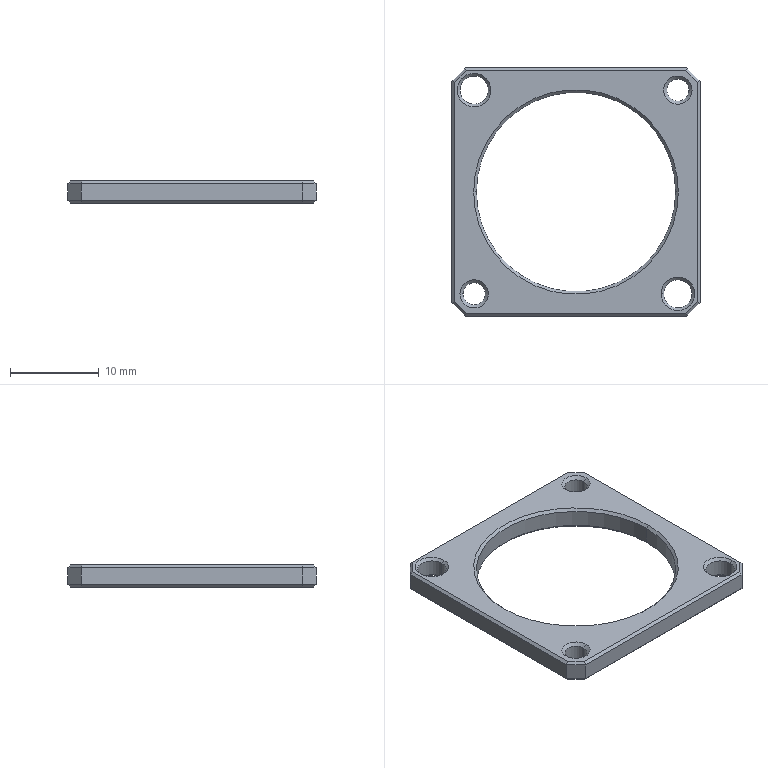Part | SolidWorks | features Chamfer 1, Extrusion 1, HoleWzd 1, ICE 1 | 1 solid | 56 faces | box 28 x 28 x 2.5 mm | volume 869.826 mm3 | plane 26 | cone 20 | cylinder 10 | commonest cylinder face diameters 2.5 x4 3.2 x4 22.5 x2
STEP:
#1=CARTESIAN_POINT('',(-11.25,0.,2.2));
#2=VERTEX_POINT('',#1);
#3=CARTESIAN_POINT('',(11.25,0.,2.2));
#4=VERTEX_POINT('',#3);
#5=CARTESIAN_POINT('',(0.,0.,2.2));
#6=DIRECTION('',(0.,0.,1.));
#7=DIRECTION('',(1.,0.,0.));
#8=AXIS2_PLACEMENT_3D('',#5,#6,#7);
#9=CIRCLE('',#8,11.25);
#10=EDGE_CURVE('',#2,#4,#9,.T.);
#11=ORIENTED_EDGE('',*,*,#10,.F.);
#12=CARTESIAN_POINT('',(-11.55,0.,2.5));
#13=VERTEX_POINT('',#12);
#14=CARTESIAN_POINT('',(-11.25,0.,2.2));
#15=DIRECTION('',(-0.7071,0.,0.7071));
#16=VECTOR('',#15,1000.);
#17=LINE('',#14,#16);
#18=EDGE_CURVE('',#2,#13,#17,.T.);
#19=ORIENTED_EDGE('',*,*,#18,.T.);
#20=CARTESIAN_POINT('',(11.55,0.,2.5));
#21=VERTEX_POINT('',#20);
#22=CARTESIAN_POINT('',(0.,0.,2.5));
#23=DIRECTION('',(0.,0.,-1.));
#24=DIRECTION('',(1.,0.,0.));
#25=AXIS2_PLACEMENT_3D('',#22,#23,#24);
#26=CIRCLE('',#25,11.55);
#27=EDGE_CURVE('',#21,#13,#26,.T.);
#28=ORIENTED_EDGE('',*,*,#27,.F.);
#29=CARTESIAN_POINT('',(11.25,0.,2.2));
#30=DIRECTION('',(0.7071,0.,0.7071));
#31=VECTOR('',#30,1000.);
#32=LINE('',#29,#31);
#33=EDGE_CURVE('',#4,#21,#32,.T.);
#34=ORIENTED_EDGE('',*,*,#33,.F.);
#35=EDGE_LOOP('',(#11,#19,#28,#34));
#36=FACE_OUTER_BOUND('',#35,.T.);
#37=CARTESIAN_POINT('',(0.,0.,2.2));
#38=DIRECTION('',(0.,0.,1.));
#39=DIRECTION('',(1.,0.,0.));
#40=AXIS2_PLACEMENT_3D('',#37,#38,#39);
#41=CONICAL_SURFACE('',#40,11.25,0.7854);
#42=ADVANCED_FACE('',(#36),#41,.F.);
#43=CARTESIAN_POINT('',(11.25,0.,0.3));
#44=VERTEX_POINT('',#43);
#45=CARTESIAN_POINT('',(-11.25,0.,0.3));
#46=VERTEX_POINT('',#45);
#47=CARTESIAN_POINT('',(0.,0.,0.3));
#48=DIRECTION('',(0.,0.,-1.));
#49=DIRECTION('',(1.,0.,0.));
#50=AXIS2_PLACEMENT_3D('',#47,#48,#49);
#51=CIRCLE('',#50,11.25);
#52=EDGE_CURVE('',#44,#46,#51,.T.);
#53=ORIENTED_EDGE('',*,*,#52,.F.);
#54=CARTESIAN_POINT('',(11.55,0.,0.));
#55=VERTEX_POINT('',#54);
#56=CARTESIAN_POINT('',(11.55,0.,0.));
#57=DIRECTION('',(0.7071,0.,-0.7071));
#58=VECTOR('',#57,1000.);
#59=LINE('',#56,#58);
#60=EDGE_CURVE('',#44,#55,#59,.T.);
#61=ORIENTED_EDGE('',*,*,#60,.T.);
#62=CARTESIAN_POINT('',(-11.55,0.,0.));
#63=VERTEX_POINT('',#62);
#64=CARTESIAN_POINT('',(0.,0.,0.));
#65=DIRECTION('',(0.,0.,1.));
#66=DIRECTION('',(1.,0.,0.));
#67=AXIS2_PLACEMENT_3D('',#64,#65,#66);
#68=CIRCLE('',#67,11.55);
#69=EDGE_CURVE('',#63,#55,#68,.T.);
#70=ORIENTED_EDGE('',*,*,#69,.F.);
#71=CARTESIAN_POINT('',(-11.55,0.,0.));
#72=DIRECTION('',(-0.7071,0.,-0.7071));
#73=VECTOR('',#72,1000.);
#74=LINE('',#71,#73);
#75=EDGE_CURVE('',#46,#63,#74,.T.);
#76=ORIENTED_EDGE('',*,*,#75,.F.);
#77=EDGE_LOOP('',(#53,#61,#70,#76));
#78=FACE_OUTER_BOUND('',#77,.T.);
#79=CARTESIAN_POINT('',(0.,0.,0.));
#80=DIRECTION('',(0.,0.,-1.));
#81=DIRECTION('',(-1.,0.,0.));
#82=AXIS2_PLACEMENT_3D('',#79,#80,#81);
#83=CONICAL_SURFACE('',#82,11.55,0.7854);
#84=ADVANCED_FACE('',(#78),#83,.F.);
#85=CARTESIAN_POINT('',(13.1,-11.5,0.3));
#86=VERTEX_POINT('',#85);
#87=CARTESIAN_POINT('',(9.9,-11.5,0.3));
#88=VERTEX_POINT('',#87);
#89=CARTESIAN_POINT('',(11.5,-11.5,0.3));
#90=DIRECTION('',(0.,0.,-1.));
#91=DIRECTION('',(1.,0.,0.));
#92=AXIS2_PLACEMENT_3D('',#89,#90,#91);
#93=CIRCLE('',#92,1.6);
#94=EDGE_CURVE('',#86,#88,#93,.T.);
#95=ORIENTED_EDGE('',*,*,#94,.F.);
#96=CARTESIAN_POINT('',(13.4,-11.5,0.));
#97=VERTEX_POINT('',#96);
#98=CARTESIAN_POINT('',(13.4,-11.5,0.));
#99=DIRECTION('',(0.7071,0.,-0.7071));
#100=VECTOR('',#99,1000.);
#101=LINE('',#98,#100);
#102=EDGE_CURVE('',#86,#97,#101,.T.);
#103=ORIENTED_EDGE('',*,*,#102,.T.);
#104=CARTESIAN_POINT('',(9.6,-11.5,0.));
#105=VERTEX_POINT('',#104);
#106=CARTESIAN_POINT('',(11.5,-11.5,0.));
#107=DIRECTION('',(0.,0.,1.));
#108=DIRECTION('',(1.,0.,0.));
#109=AXIS2_PLACEMENT_3D('',#106,#107,#108);
#110=CIRCLE('',#109,1.9);
#111=EDGE_CURVE('',#105,#97,#110,.T.);
#112=ORIENTED_EDGE('',*,*,#111,.F.);
#113=CARTESIAN_POINT('',(9.6,-11.5,0.));
#114=DIRECTION('',(-0.7071,0.,-0.7071));
#115=VECTOR('',#114,1000.);
#116=LINE('',#113,#115);
#117=EDGE_CURVE('',#88,#105,#116,.T.);
#118=ORIENTED_EDGE('',*,*,#117,.F.);
#119=EDGE_LOOP('',(#95,#103,#112,#118));
#120=FACE_OUTER_BOUND('',#119,.T.);
#121=CARTESIAN_POINT('',(11.5,-11.5,0.));
#122=DIRECTION('',(0.,0.,-1.));
#123=DIRECTION('',(-1.,0.,0.));
#124=AXIS2_PLACEMENT_3D('',#121,#122,#123);
#125=CONICAL_SURFACE('',#124,1.9,0.7854);
#126=ADVANCED_FACE('',(#120),#125,.F.);
#127=CARTESIAN_POINT('',(9.9,-11.5,2.2));
#128=VERTEX_POINT('',#127);
#129=CARTESIAN_POINT('',(13.1,-11.5,2.2));
#130=VERTEX_POINT('',#129);
#131=CARTESIAN_POINT('',(11.5,-11.5,2.2));
#132=DIRECTION('',(0.,0.,1.));
#133=DIRECTION('',(1.,0.,0.));
#134=AXIS2_PLACEMENT_3D('',#131,#132,#133);
#135=CIRCLE('',#134,1.6);
#136=EDGE_CURVE('',#128,#130,#135,.T.);
#137=ORIENTED_EDGE('',*,*,#136,.F.);
#138=CARTESIAN_POINT('',(9.6,-11.5,2.5));
#139=VERTEX_POINT('',#138);
#140=CARTESIAN_POINT('',(9.9,-11.5,2.2));
#141=DIRECTION('',(-0.7071,0.,0.7071));
#142=VECTOR('',#141,1000.);
#143=LINE('',#140,#142);
#144=EDGE_CURVE('',#128,#139,#143,.T.);
#145=ORIENTED_EDGE('',*,*,#144,.T.);
#146=CARTESIAN_POINT('',(13.4,-11.5,2.5));
#147=VERTEX_POINT('',#146);
#148=CARTESIAN_POINT('',(11.5,-11.5,2.5));
#149=DIRECTION('',(0.,0.,-1.));
#150=DIRECTION('',(1.,0.,0.));
#151=AXIS2_PLACEMENT_3D('',#148,#149,#150);
#152=CIRCLE('',#151,1.9);
#153=EDGE_CURVE('',#147,#139,#152,.T.);
#154=ORIENTED_EDGE('',*,*,#153,.F.);
#155=CARTESIAN_POINT('',(13.1,-11.5,2.2));
#156=DIRECTION('',(0.7071,0.,0.7071));
#157=VECTOR('',#156,1000.);
#158=LINE('',#155,#157);
#159=EDGE_CURVE('',#130,#147,#158,.T.);
#160=ORIENTED_EDGE('',*,*,#159,.F.);
#161=EDGE_LOOP('',(#137,#145,#154,#160));
#162=FACE_OUTER_BOUND('',#161,.T.);
#163=CARTESIAN_POINT('',(11.5,-11.5,2.2));
#164=DIRECTION('',(0.,0.,1.));
#165=DIRECTION('',(1.,0.,0.));
#166=AXIS2_PLACEMENT_3D('',#163,#164,#165);
#167=CONICAL_SURFACE('',#166,1.6,0.7854);
#168=ADVANCED_FACE('',(#162),#167,.F.);
#169=CARTESIAN_POINT('',(-9.9,11.5,0.3));
#170=VERTEX_POINT('',#169);
#171=CARTESIAN_POINT('',(-13.1,11.5,0.3));
#172=VERTEX_POINT('',#171);
#173=CARTESIAN_POINT('',(-11.5,11.5,0.3));
#174=DIRECTION('',(0.,0.,-1.));
#175=DIRECTION('',(1.,0.,0.));
#176=AXIS2_PLACEMENT_3D('',#173,#174,#175);
#177=CIRCLE('',#176,1.6);
#178=EDGE_CURVE('',#170,#172,#177,.T.);
#179=ORIENTED_EDGE('',*,*,#178,.F.);
#180=CARTESIAN_POINT('',(-9.6,11.5,0.));
#181=VERTEX_POINT('',#180);
#182=CARTESIAN_POINT('',(-9.6,11.5,0.));
#183=DIRECTION('',(0.7071,0.,-0.7071));
#184=VECTOR('',#183,1000.);
#185=LINE('',#182,#184);
#186=EDGE_CURVE('',#170,#181,#185,.T.);
#187=ORIENTED_EDGE('',*,*,#186,.T.);
#188=CARTESIAN_POINT('',(-13.4,11.5,0.));
#189=VERTEX_POINT('',#188);
#190=CARTESIAN_POINT('',(-11.5,11.5,0.));
#191=DIRECTION('',(0.,0.,1.));
#192=DIRECTION('',(1.,0.,0.));
#193=AXIS2_PLACEMENT_3D('',#190,#191,#192);
#194=CIRCLE('',#193,1.9);
#195=EDGE_CURVE('',#189,#181,#194,.T.);
#196=ORIENTED_EDGE('',*,*,#195,.F.);
#197=CARTESIAN_POINT('',(-13.4,11.5,0.));
#198=DIRECTION('',(-0.7071,0.,-0.7071));
#199=VECTOR('',#198,1000.);
#200=LINE('',#197,#199);
#201=EDGE_CURVE('',#172,#189,#200,.T.);
#202=ORIENTED_EDGE('',*,*,#201,.F.);
#203=EDGE_LOOP('',(#179,#187,#196,#202));
#204=FACE_OUTER_BOUND('',#203,.T.);
#205=CARTESIAN_POINT('',(-11.5,11.5,0.));
#206=DIRECTION('',(0.,0.,-1.));
#207=DIRECTION('',(-1.,0.,0.));
#208=AXIS2_PLACEMENT_3D('',#205,#206,#207);
#209=CONICAL_SURFACE('',#208,1.9,0.7854);
#210=ADVANCED_FACE('',(#204),#209,.F.);
#211=CARTESIAN_POINT('',(-13.1,11.5,2.2));
#212=VERTEX_POINT('',#211);
#213=CARTESIAN_POINT('',(-9.9,11.5,2.2));
#214=VERTEX_POINT('',#213);
#215=CARTESIAN_POINT('',(-11.5,11.5,2.2));
#216=DIRECTION('',(0.,0.,1.));
#217=DIRECTION('',(1.,0.,0.));
#218=AXIS2_PLACEMENT_3D('',#215,#216,#217);
#219=CIRCLE('',#218,1.6);
#220=EDGE_CURVE('',#212,#214,#219,.T.);
#221=ORIENTED_EDGE('',*,*,#220,.F.);
#222=CARTESIAN_POINT('',(-13.4,11.5,2.5));
#223=VERTEX_POINT('',#222);
#224=CARTESIAN_POINT('',(-13.1,11.5,2.2));
#225=DIRECTION('',(-0.7071,0.,0.7071));
#226=VECTOR('',#225,1000.);
#227=LINE('',#224,#226);
#228=EDGE_CURVE('',#212,#223,#227,.T.);
#229=ORIENTED_EDGE('',*,*,#228,.T.);
#230=CARTESIAN_POINT('',(-9.6,11.5,2.5));
#231=VERTEX_POINT('',#230);
#232=CARTESIAN_POINT('',(-11.5,11.5,2.5));
#233=DIRECTION('',(0.,0.,-1.));
#234=DIRECTION('',(1.,0.,0.));
#235=AXIS2_PLACEMENT_3D('',#232,#233,#234);
#236=CIRCLE('',#235,1.9);
#237=EDGE_CURVE('',#231,#223,#236,.T.);
#238=ORIENTED_EDGE('',*,*,#237,.F.);
#239=CARTESIAN_POINT('',(-9.9,11.5,2.2));
#240=DIRECTION('',(0.7071,0.,0.7071));
#241=VECTOR('',#240,1000.);
#242=LINE('',#239,#241);
#243=EDGE_CURVE('',#214,#231,#242,.T.);
#244=ORIENTED_EDGE('',*,*,#243,.F.);
#245=EDGE_LOOP('',(#221,#229,#238,#244));
#246=FACE_OUTER_BOUND('',#245,.T.);
#247=CARTESIAN_POINT('',(-11.5,11.5,2.2));
#248=DIRECTION('',(0.,0.,1.));
#249=DIRECTION('',(1.,0.,0.));
#250=AXIS2_PLACEMENT_3D('',#247,#248,#249);
#251=CONICAL_SURFACE('',#250,1.6,0.7854);
#252=ADVANCED_FACE('',(#246),#251,.F.);
#253=CARTESIAN_POINT('',(-12.75,-11.5,2.15));
#254=VERTEX_POINT('',#253);
#255=CARTESIAN_POINT('',(-10.25,-11.5,2.15));
#256=VERTEX_POINT('',#255);
#257=CARTESIAN_POINT('',(-11.5,-11.5,2.15));
#258=DIRECTION('',(0.,0.,1.));
#259=DIRECTION('',(1.,0.,0.));
#260=AXIS2_PLACEMENT_3D('',#257,#258,#259);
#261=CIRCLE('',#260,1.25);
#262=EDGE_CURVE('',#254,#256,#261,.T.);
#263=ORIENTED_EDGE('',*,*,#262,.F.);
#264=CARTESIAN_POINT('',(-13.1,-11.5,2.5));
#265=VERTEX_POINT('',#264);
#266=CARTESIAN_POINT('',(-13.1,-11.5,2.5));
#267=DIRECTION('',(-0.7071,0.,0.7071));
#268=VECTOR('',#267,1000.);
#269=LINE('',#266,#268);
#270=EDGE_CURVE('',#254,#265,#269,.T.);
#271=ORIENTED_EDGE('',*,*,#270,.T.);
#272=CARTESIAN_POINT('',(-9.9,-11.5,2.5));
#273=VERTEX_POINT('',#272);
#274=CARTESIAN_POINT('',(-11.5,-11.5,2.5));
#275=DIRECTION('',(0.,0.,1.));
#276=DIRECTION('',(1.,0.,0.));
#277=AXIS2_PLACEMENT_3D('',#274,#275,#276);
#278=CIRCLE('',#277,1.6);
#279=EDGE_CURVE('',#265,#273,#278,.T.);
#280=ORIENTED_EDGE('',*,*,#279,.T.);
#281=CARTESIAN_POINT('',(-9.9,-11.5,2.5));
#282=DIRECTION('',(0.7071,0.,0.7071));
#283=VECTOR('',#282,1000.);
#284=LINE('',#281,#283);
#285=EDGE_CURVE('',#256,#273,#284,.T.);
#286=ORIENTED_EDGE('',*,*,#285,.F.);
#287=EDGE_LOOP('',(#263,#271,#280,#286));
#288=FACE_OUTER_BOUND('',#287,.T.);
#289=CARTESIAN_POINT('',(-11.5,-11.5,2.5));
#290=DIRECTION('',(0.,0.,1.));
#291=DIRECTION('',(1.,0.,0.));
#292=AXIS2_PLACEMENT_3D('',#289,#290,#291);
#293=CONICAL_SURFACE('',#292,1.6,0.7854);
#294=ADVANCED_FACE('',(#288),#293,.F.);
#295=CARTESIAN_POINT('',(-12.75,-11.5,0.35));
#296=VERTEX_POINT('',#295);
#297=CARTESIAN_POINT('',(-10.25,-11.5,0.35));
#298=VERTEX_POINT('',#297);
#299=CARTESIAN_POINT('',(-11.5,-11.5,0.35));
#300=DIRECTION('',(0.,0.,1.));
#301=DIRECTION('',(1.,0.,0.));
#302=AXIS2_PLACEMENT_3D('',#299,#300,#301);
#303=CIRCLE('',#302,1.25);
#304=EDGE_CURVE('',#296,#298,#303,.T.);
#305=ORIENTED_EDGE('',*,*,#304,.F.);
#306=CARTESIAN_POINT('',(-12.75,-11.5,2.5));
#307=DIRECTION('',(0.,0.,1.));
#308=VECTOR('',#307,1000.);
#309=LINE('',#306,#308);
#310=EDGE_CURVE('',#296,#254,#309,.T.);
#311=ORIENTED_EDGE('',*,*,#310,.T.);
#312=ORIENTED_EDGE('',*,*,#262,.T.);
#313=CARTESIAN_POINT('',(-10.25,-11.5,2.5));
#314=DIRECTION('',(0.,0.,1.));
#315=VECTOR('',#314,1000.);
#316=LINE('',#313,#315);
#317=EDGE_CURVE('',#298,#256,#316,.T.);
#318=ORIENTED_EDGE('',*,*,#317,.F.);
#319=EDGE_LOOP('',(#305,#311,#312,#318));
#320=FACE_OUTER_BOUND('',#319,.T.);
#321=CARTESIAN_POINT('',(-11.5,-11.5,2.5));
#322=DIRECTION('',(0.,0.,1.));
#323=DIRECTION('',(1.,0.,0.));
#324=AXIS2_PLACEMENT_3D('',#321,#322,#323);
#325=CYLINDRICAL_SURFACE('',#324,1.25);
#326=ADVANCED_FACE('',(#320),#325,.F.);
#327=ORIENTED_EDGE('',*,*,#304,.T.);
#328=CARTESIAN_POINT('',(-9.9,-11.5,0.));
#329=VERTEX_POINT('',#328);
#330=CARTESIAN_POINT('',(-10.25,-11.5,0.35));
#331=DIRECTION('',(0.7071,0.,-0.7071));
#332=VECTOR('',#331,1000.);
#333=LINE('',#330,#332);
#334=EDGE_CURVE('',#298,#329,#333,.T.);
#335=ORIENTED_EDGE('',*,*,#334,.T.);
#336=CARTESIAN_POINT('',(-13.1,-11.5,0.));
#337=VERTEX_POINT('',#336);
#338=CARTESIAN_POINT('',(-11.5,-11.5,0.));
#339=DIRECTION('',(0.,0.,1.));
#340=DIRECTION('',(1.,0.,0.));
#341=AXIS2_PLACEMENT_3D('',#338,#339,#340);
#342=CIRCLE('',#341,1.6);
#343=EDGE_CURVE('',#337,#329,#342,.T.);
#344=ORIENTED_EDGE('',*,*,#343,.F.);
#345=CARTESIAN_POINT('',(-12.75,-11.5,0.35));
#346=DIRECTION('',(-0.7071,0.,-0.7071));
#347=VECTOR('',#346,1000.);
#348=LINE('',#345,#347);
#349=EDGE_CURVE('',#296,#337,#348,.T.);
#350=ORIENTED_EDGE('',*,*,#349,.F.);
#351=EDGE_LOOP('',(#327,#335,#344,#350));
#352=FACE_OUTER_BOUND('',#351,.T.);
#353=CARTESIAN_POINT('',(-11.5,-11.5,0.35));
#354=DIRECTION('',(0.,0.,-1.));
#355=DIRECTION('',(-1.,0.,0.));
#356=AXIS2_PLACEMENT_3D('',#353,#354,#355);
#357=CONICAL_SURFACE('',#356,1.25,0.7854);
#358=ADVANCED_FACE('',(#352),#357,.F.);
#359=CARTESIAN_POINT('',(10.25,11.5,2.15));
#360=VERTEX_POINT('',#359);
#361=CARTESIAN_POINT('',(12.75,11.5,2.15));
#362=VERTEX_POINT('',#361);
#363=CARTESIAN_POINT('',(11.5,11.5,2.15));
#364=DIRECTION('',(0.,0.,1.));
#365=DIRECTION('',(1.,0.,0.));
#366=AXIS2_PLACEMENT_3D('',#363,#364,#365);
#367=CIRCLE('',#366,1.25);
#368=EDGE_CURVE('',#360,#362,#367,.T.);
#369=ORIENTED_EDGE('',*,*,#368,.F.);
#370=CARTESIAN_POINT('',(9.9,11.5,2.5));
#371=VERTEX_POINT('',#370);
#372=CARTESIAN_POINT('',(9.9,11.5,2.5));
#373=DIRECTION('',(-0.7071,0.,0.7071));
#374=VECTOR('',#373,1000.);
#375=LINE('',#372,#374);
#376=EDGE_CURVE('',#360,#371,#375,.T.);
#377=ORIENTED_EDGE('',*,*,#376,.T.);
#378=CARTESIAN_POINT('',(13.1,11.5,2.5));
#379=VERTEX_POINT('',#378);
#380=CARTESIAN_POINT('',(11.5,11.5,2.5));
#381=DIRECTION('',(0.,0.,1.));
#382=DIRECTION('',(1.,0.,0.));
#383=AXIS2_PLACEMENT_3D('',#380,#381,#382);
#384=CIRCLE('',#383,1.6);
#385=EDGE_CURVE('',#371,#379,#384,.T.);
#386=ORIENTED_EDGE('',*,*,#385,.T.);
#387=CARTESIAN_POINT('',(13.1,11.5,2.5));
#388=DIRECTION('',(0.7071,0.,0.7071));
#389=VECTOR('',#388,1000.);
#390=LINE('',#387,#389);
#391=EDGE_CURVE('',#362,#379,#390,.T.);
#392=ORIENTED_EDGE('',*,*,#391,.F.);
#393=EDGE_LOOP('',(#369,#377,#386,#392));
#394=FACE_OUTER_BOUND('',#393,.T.);
#395=CARTESIAN_POINT('',(11.5,11.5,2.5));
#396=DIRECTION('',(0.,0.,1.));
#397=DIRECTION('',(1.,0.,0.));
#398=AXIS2_PLACEMENT_3D('',#395,#396,#397);
#399=CONICAL_SURFACE('',#398,1.6,0.7854);
#400=ADVANCED_FACE('',(#394),#399,.F.);
#401=CARTESIAN_POINT('',(10.25,11.5,0.35));
#402=VERTEX_POINT('',#401);
#403=CARTESIAN_POINT('',(12.75,11.5,0.35));
#404=VERTEX_POINT('',#403);
#405=CARTESIAN_POINT('',(11.5,11.5,0.35));
#406=DIRECTION('',(0.,0.,1.));
#407=DIRECTION('',(1.,0.,0.));
#408=AXIS2_PLACEMENT_3D('',#405,#406,#407);
#409=CIRCLE('',#408,1.25);
#410=EDGE_CURVE('',#402,#404,#409,.T.);
#411=ORIENTED_EDGE('',*,*,#410,.F.);
#412=CARTESIAN_POINT('',(10.25,11.5,2.5));
#413=DIRECTION('',(0.,0.,1.));
#414=VECTOR('',#413,1000.);
#415=LINE('',#412,#414);
#416=EDGE_CURVE('',#402,#360,#415,.T.);
#417=ORIENTED_EDGE('',*,*,#416,.T.);
#418=ORIENTED_EDGE('',*,*,#368,.T.);
#419=CARTESIAN_POINT('',(12.75,11.5,2.5));
#420=DIRECTION('',(0.,0.,1.));
#421=VECTOR('',#420,1000.);
#422=LINE('',#419,#421);
#423=EDGE_CURVE('',#404,#362,#422,.T.);
#424=ORIENTED_EDGE('',*,*,#423,.F.);
#425=EDGE_LOOP('',(#411,#417,#418,#424));
#426=FACE_OUTER_BOUND('',#425,.T.);
#427=CARTESIAN_POINT('',(11.5,11.5,2.5));
#428=DIRECTION('',(0.,0.,1.));
#429=DIRECTION('',(1.,0.,0.));
#430=AXIS2_PLACEMENT_3D('',#427,#428,#429);
#431=CYLINDRICAL_SURFACE('',#430,1.25);
#432=ADVANCED_FACE('',(#426),#431,.F.);
#433=ORIENTED_EDGE('',*,*,#410,.T.);
#434=CARTESIAN_POINT('',(13.1,11.5,0.));
#435=VERTEX_POINT('',#434);
#436=CARTESIAN_POINT('',(12.75,11.5,0.35));
#437=DIRECTION('',(0.7071,0.,-0.7071));
#438=VECTOR('',#437,1000.);
#439=LINE('',#436,#438);
#440=EDGE_CURVE('',#404,#435,#439,.T.);
#441=ORIENTED_EDGE('',*,*,#440,.T.);
#442=CARTESIAN_POINT('',(9.9,11.5,0.));
#443=VERTEX_POINT('',#442);
#444=CARTESIAN_POINT('',(11.5,11.5,0.));
#445=DIRECTION('',(0.,0.,1.));
#446=DIRECTION('',(1.,0.,0.));
#447=AXIS2_PLACEMENT_3D('',#444,#445,#446);
#448=CIRCLE('',#447,1.6);
#449=EDGE_CURVE('',#443,#435,#448,.T.);
#450=ORIENTED_EDGE('',*,*,#449,.F.);
#451=CARTESIAN_POINT('',(10.25,11.5,0.35));
#452=DIRECTION('',(-0.7071,0.,-0.7071));
#453=VECTOR('',#452,1000.);
#454=LINE('',#451,#453);
#455=EDGE_CURVE('',#402,#443,#454,.T.);
#456=ORIENTED_EDGE('',*,*,#455,.F.);
#457=EDGE_LOOP('',(#433,#441,#450,#456));
#458=FACE_OUTER_BOUND('',#457,.T.);
#459=CARTESIAN_POINT('',(11.5,11.5,0.35));
#460=DIRECTION('',(0.,0.,-1.));
#461=DIRECTION('',(-1.,0.,0.));
#462=AXIS2_PLACEMENT_3D('',#459,#460,#461);
#463=CONICAL_SURFACE('',#462,1.25,0.7854);
#464=ADVANCED_FACE('',(#458),#463,.F.);
#465=ORIENTED_EDGE('',*,*,#178,.T.);
#466=CARTESIAN_POINT('',(-13.1,11.5,0.));
#467=DIRECTION('',(0.,0.,1.));
#468=VECTOR('',#467,1000.);
#469=LINE('',#466,#468);
#470=EDGE_CURVE('',#172,#212,#469,.T.);
#471=ORIENTED_EDGE('',*,*,#470,.T.);
#472=ORIENTED_EDGE('',*,*,#220,.T.);
#473=CARTESIAN_POINT('',(-9.9,11.5,0.));
#474=DIRECTION('',(0.,0.,1.));
#475=VECTOR('',#474,1000.);
#476=LINE('',#473,#475);
#477=EDGE_CURVE('',#170,#214,#476,.T.);
#478=ORIENTED_EDGE('',*,*,#477,.F.);
#479=EDGE_LOOP('',(#465,#471,#472,#478));
#480=FACE_OUTER_BOUND('',#479,.T.);
#481=CARTESIAN_POINT('',(-11.5,11.5,0.));
#482=DIRECTION('',(0.,0.,1.));
#483=DIRECTION('',(1.,0.,0.));
#484=AXIS2_PLACEMENT_3D('',#481,#482,#483);
#485=CYLINDRICAL_SURFACE('',#484,1.6);
#486=ADVANCED_FACE('',(#480),#485,.F.);
#487=ORIENTED_EDGE('',*,*,#94,.T.);
#488=CARTESIAN_POINT('',(9.9,-11.5,0.));
#489=DIRECTION('',(0.,0.,1.));
#490=VECTOR('',#489,1000.);
#491=LINE('',#488,#490);
#492=EDGE_CURVE('',#88,#128,#491,.T.);
#493=ORIENTED_EDGE('',*,*,#492,.T.);
#494=ORIENTED_EDGE('',*,*,#136,.T.);
#495=CARTESIAN_POINT('',(13.1,-11.5,0.));
#496=DIRECTION('',(0.,0.,1.));
#497=VECTOR('',#496,1000.);
#498=LINE('',#495,#497);
#499=EDGE_CURVE('',#86,#130,#498,.T.);
#500=ORIENTED_EDGE('',*,*,#499,.F.);
#501=EDGE_LOOP('',(#487,#493,#494,#500));
#502=FACE_OUTER_BOUND('',#501,.T.);
#503=CARTESIAN_POINT('',(11.5,-11.5,0.));
#504=DIRECTION('',(0.,0.,1.));
#505=DIRECTION('',(1.,0.,0.));
#506=AXIS2_PLACEMENT_3D('',#503,#504,#505);
#507=CYLINDRICAL_SURFACE('',#506,1.6);
#508=ADVANCED_FACE('',(#502),#507,.F.);
#509=ORIENTED_EDGE('',*,*,#10,.T.);
#510=CARTESIAN_POINT('',(11.25,0.,2.5));
#511=DIRECTION('',(0.,0.,-1.));
#512=VECTOR('',#511,1000.);
#513=LINE('',#510,#512);
#514=EDGE_CURVE('',#4,#44,#513,.T.);
#515=ORIENTED_EDGE('',*,*,#514,.T.);
#516=ORIENTED_EDGE('',*,*,#52,.T.);
#517=CARTESIAN_POINT('',(-11.25,0.,2.5));
#518=DIRECTION('',(0.,0.,-1.));
#519=VECTOR('',#518,1000.);
#520=LINE('',#517,#519);
#521=EDGE_CURVE('',#2,#46,#520,.T.);
#522=ORIENTED_EDGE('',*,*,#521,.F.);
#523=EDGE_LOOP('',(#509,#515,#516,#522));
#524=FACE_OUTER_BOUND('',#523,.T.);
#525=CARTESIAN_POINT('',(0.,0.,2.5));
#526=DIRECTION('',(0.,0.,-1.));
#527=DIRECTION('',(-1.,0.,0.));
#528=AXIS2_PLACEMENT_3D('',#525,#526,#527);
#529=CYLINDRICAL_SURFACE('',#528,11.25);
#530=ADVANCED_FACE('',(#524),#529,.F.);
#531=ORIENTED_EDGE('',*,*,#237,.T.);
#532=CARTESIAN_POINT('',(-11.5,11.5,2.5));
#533=DIRECTION('',(0.,0.,-1.));
#534=DIRECTION('',(1.,0.,0.));
#535=AXIS2_PLACEMENT_3D('',#532,#533,#534);
#536=CIRCLE('',#535,1.9);
#537=EDGE_CURVE('',#223,#231,#536,.T.);
#538=ORIENTED_EDGE('',*,*,#537,.T.);
#539=EDGE_LOOP('',(#531,#538));
#540=FACE_BOUND('',#539,.T.);
#541=ORIENTED_EDGE('',*,*,#153,.T.);
#542=CARTESIAN_POINT('',(11.5,-11.5,2.5));
#543=DIRECTION('',(0.,0.,-1.));
#544=DIRECTION('',(1.,0.,0.));
#545=AXIS2_PLACEMENT_3D('',#542,#543,#544);
#546=CIRCLE('',#545,1.9);
#547=EDGE_CURVE('',#139,#147,#546,.T.);
#548=ORIENTED_EDGE('',*,*,#547,.T.);
#549=EDGE_LOOP('',(#541,#548));
#550=FACE_BOUND('',#549,.T.);
#551=ORIENTED_EDGE('',*,*,#27,.T.);
#552=CARTESIAN_POINT('',(0.,0.,2.5));
#553=DIRECTION('',(0.,0.,-1.));
#554=DIRECTION('',(1.,0.,0.));
#555=AXIS2_PLACEMENT_3D('',#552,#553,#554);
#556=CIRCLE('',#555,11.55);
#557=EDGE_CURVE('',#13,#21,#556,.T.);
#558=ORIENTED_EDGE('',*,*,#557,.T.);
#559=EDGE_LOOP('',(#551,#558));
#560=FACE_BOUND('',#559,.T.);
#561=CARTESIAN_POINT('',(-13.7,12.376,2.5));
#562=VERTEX_POINT('',#561);
#563=CARTESIAN_POINT('',(-13.7,-12.376,2.5));
#564=VERTEX_POINT('',#563);
#565=CARTESIAN_POINT('',(-13.7,-12.5,2.5));
#566=DIRECTION('',(0.,-1.,0.));
#567=VECTOR('',#566,1000.);
#568=LINE('',#565,#567);
#569=EDGE_CURVE('',#562,#564,#568,.T.);
#570=ORIENTED_EDGE('',*,*,#569,.T.);
#571=CARTESIAN_POINT('',(-12.376,-13.7,2.5));
#572=VERTEX_POINT('',#571);
#573=CARTESIAN_POINT('',(-12.288,-13.788,2.5));
#574=DIRECTION('',(0.7071,-0.7071,0.));
#575=VECTOR('',#574,1000.);
#576=LINE('',#573,#575);
#577=EDGE_CURVE('',#564,#572,#576,.T.);
#578=ORIENTED_EDGE('',*,*,#577,.T.);
#579=CARTESIAN_POINT('',(12.376,-13.7,2.5));
#580=VERTEX_POINT('',#579);
#581=CARTESIAN_POINT('',(12.5,-13.7,2.5));
#582=DIRECTION('',(1.,0.,0.));
#583=VECTOR('',#582,1000.);
#584=LINE('',#581,#583);
#585=EDGE_CURVE('',#572,#580,#584,.T.);
#586=ORIENTED_EDGE('',*,*,#585,.T.);
#587=CARTESIAN_POINT('',(13.7,-12.376,2.5));
#588=VERTEX_POINT('',#587);
#589=CARTESIAN_POINT('',(13.788,-12.288,2.5));
#590=DIRECTION('',(0.7071,0.7071,0.));
#591=VECTOR('',#590,1000.);
#592=LINE('',#589,#591);
#593=EDGE_CURVE('',#580,#588,#592,.T.);
#594=ORIENTED_EDGE('',*,*,#593,.T.);
#595=CARTESIAN_POINT('',(13.7,12.376,2.5));
#596=VERTEX_POINT('',#595);
#597=CARTESIAN_POINT('',(13.7,12.5,2.5));
#598=DIRECTION('',(0.,1.,0.));
#599=VECTOR('',#598,1000.);
#600=LINE('',#597,#599);
#601=EDGE_CURVE('',#588,#596,#600,.T.);
#602=ORIENTED_EDGE('',*,*,#601,.T.);
#603=CARTESIAN_POINT('',(12.376,13.7,2.5));
#604=VERTEX_POINT('',#603);
#605=CARTESIAN_POINT('',(12.288,13.788,2.5));
#606=DIRECTION('',(-0.7071,0.7071,0.));
#607=VECTOR('',#606,1000.);
#608=LINE('',#605,#607);
#609=EDGE_CURVE('',#596,#604,#608,.T.);
#610=ORIENTED_EDGE('',*,*,#609,.T.);
#611=CARTESIAN_POINT('',(-12.376,13.7,2.5));
#612=VERTEX_POINT('',#611);
#613=CARTESIAN_POINT('',(-12.5,13.7,2.5));
#614=DIRECTION('',(-1.,0.,0.));
#615=VECTOR('',#614,1000.);
#616=LINE('',#613,#615);
#617=EDGE_CURVE('',#604,#612,#616,.T.);
#618=ORIENTED_EDGE('',*,*,#617,.T.);
#619=CARTESIAN_POINT('',(-13.788,12.288,2.5));
#620=DIRECTION('',(-0.7071,-0.7071,0.));
#621=VECTOR('',#620,1000.);
#622=LINE('',#619,#621);
#623=EDGE_CURVE('',#612,#562,#622,.T.);
#624=ORIENTED_EDGE('',*,*,#623,.T.);
#625=EDGE_LOOP('',(#570,#578,#586,#594,#602,#610,#618,#624));
#626=FACE_OUTER_BOUND('',#625,.T.);
#627=CARTESIAN_POINT('',(-11.5,-11.5,2.5));
#628=DIRECTION('',(0.,0.,1.));
#629=DIRECTION('',(1.,0.,0.));
#630=AXIS2_PLACEMENT_3D('',#627,#628,#629);
#631=CIRCLE('',#630,1.6);
#632=EDGE_CURVE('',#273,#265,#631,.T.);
#633=ORIENTED_EDGE('',*,*,#632,.F.);
#634=ORIENTED_EDGE('',*,*,#279,.F.);
#635=EDGE_LOOP('',(#633,#634));
#636=FACE_BOUND('',#635,.T.);
#637=CARTESIAN_POINT('',(11.5,11.5,2.5));
#638=DIRECTION('',(0.,0.,1.));
#639=DIRECTION('',(1.,0.,0.));
#640=AXIS2_PLACEMENT_3D('',#637,#638,#639);
#641=CIRCLE('',#640,1.6);
#642=EDGE_CURVE('',#379,#371,#641,.T.);
#643=ORIENTED_EDGE('',*,*,#642,.F.);
#644=ORIENTED_EDGE('',*,*,#385,.F.);
#645=EDGE_LOOP('',(#643,#644));
#646=FACE_BOUND('',#645,.T.);
#647=CARTESIAN_POINT('',(0.,0.,2.5));
#648=DIRECTION('',(0.,0.,1.));
#649=DIRECTION('',(1.,0.,0.));
#650=AXIS2_PLACEMENT_3D('',#647,#648,#649);
#651=PLANE('',#650);
#652=ADVANCED_FACE('',(#540,#550,#560,#626,#636,#646),#651,.T.);
#653=ORIENTED_EDGE('',*,*,#195,.T.);
#654=CARTESIAN_POINT('',(-11.5,11.5,0.));
#655=DIRECTION('',(0.,0.,1.));
#656=DIRECTION('',(1.,0.,0.));
#657=AXIS2_PLACEMENT_3D('',#654,#655,#656);
#658=CIRCLE('',#657,1.9);
#659=EDGE_CURVE('',#181,#189,#658,.T.);
#660=ORIENTED_EDGE('',*,*,#659,.T.);
#661=EDGE_LOOP('',(#653,#660));
#662=FACE_BOUND('',#661,.T.);
#663=ORIENTED_EDGE('',*,*,#111,.T.);
#664=CARTESIAN_POINT('',(11.5,-11.5,0.));
#665=DIRECTION('',(0.,0.,1.));
#666=DIRECTION('',(1.,0.,0.));
#667=AXIS2_PLACEMENT_3D('',#664,#665,#666);
#668=CIRCLE('',#667,1.9);
#669=EDGE_CURVE('',#97,#105,#668,.T.);
#670=ORIENTED_EDGE('',*,*,#669,.T.);
#671=EDGE_LOOP('',(#663,#670));
#672=FACE_BOUND('',#671,.T.);
#673=CARTESIAN_POINT('',(12.376,-13.7,0.));
#674=VERTEX_POINT('',#673);
#675=CARTESIAN_POINT('',(-12.376,-13.7,0.));
#676=VERTEX_POINT('',#675);
#677=CARTESIAN_POINT('',(0.,-13.7,0.));
#678=DIRECTION('',(-1.,0.,0.));
#679=VECTOR('',#678,1000.);
#680=LINE('',#677,#679);
#681=EDGE_CURVE('',#674,#676,#680,.T.);
#682=ORIENTED_EDGE('',*,*,#681,.T.);
#683=CARTESIAN_POINT('',(-13.7,-12.376,0.));
#684=VERTEX_POINT('',#683);
#685=CARTESIAN_POINT('',(-13.038,-13.038,0.));
#686=DIRECTION('',(-0.7071,0.7071,0.));
#687=VECTOR('',#686,1000.);
#688=LINE('',#685,#687);
#689=EDGE_CURVE('',#676,#684,#688,.T.);
#690=ORIENTED_EDGE('',*,*,#689,.T.);
#691=CARTESIAN_POINT('',(-13.7,12.376,0.));
#692=VERTEX_POINT('',#691);
#693=CARTESIAN_POINT('',(-13.7,0.,0.));
#694=DIRECTION('',(0.,1.,0.));
#695=VECTOR('',#694,1000.);
#696=LINE('',#693,#695);
#697=EDGE_CURVE('',#684,#692,#696,.T.);
#698=ORIENTED_EDGE('',*,*,#697,.T.);
#699=CARTESIAN_POINT('',(-12.376,13.7,0.));
#700=VERTEX_POINT('',#699);
#701=CARTESIAN_POINT('',(-13.038,13.038,0.));
#702=DIRECTION('',(0.7071,0.7071,0.));
#703=VECTOR('',#702,1000.);
#704=LINE('',#701,#703);
#705=EDGE_CURVE('',#692,#700,#704,.T.);
#706=ORIENTED_EDGE('',*,*,#705,.T.);
#707=CARTESIAN_POINT('',(12.376,13.7,0.));
#708=VERTEX_POINT('',#707);
#709=CARTESIAN_POINT('',(0.,13.7,0.));
#710=DIRECTION('',(1.,0.,0.));
#711=VECTOR('',#710,1000.);
#712=LINE('',#709,#711);
#713=EDGE_CURVE('',#700,#708,#712,.T.);
#714=ORIENTED_EDGE('',*,*,#713,.T.);
#715=CARTESIAN_POINT('',(13.7,12.376,0.));
#716=VERTEX_POINT('',#715);
#717=CARTESIAN_POINT('',(13.038,13.038,0.));
#718=DIRECTION('',(0.7071,-0.7071,0.));
#719=VECTOR('',#718,1000.);
#720=LINE('',#717,#719);
#721=EDGE_CURVE('',#708,#716,#720,.T.);
#722=ORIENTED_EDGE('',*,*,#721,.T.);
#723=CARTESIAN_POINT('',(13.7,-12.376,0.));
#724=VERTEX_POINT('',#723);
#725=CARTESIAN_POINT('',(13.7,0.,0.));
#726=DIRECTION('',(0.,-1.,0.));
#727=VECTOR('',#726,1000.);
#728=LINE('',#725,#727);
#729=EDGE_CURVE('',#716,#724,#728,.T.);
#730=ORIENTED_EDGE('',*,*,#729,.T.);
#731=CARTESIAN_POINT('',(13.038,-13.038,0.));
#732=DIRECTION('',(-0.7071,-0.7071,0.));
#733=VECTOR('',#732,1000.);
#734=LINE('',#731,#733);
#735=EDGE_CURVE('',#724,#674,#734,.T.);
#736=ORIENTED_EDGE('',*,*,#735,.T.);
#737=EDGE_LOOP('',(#682,#690,#698,#706,#714,#722,#730,#736));
#738=FACE_OUTER_BOUND('',#737,.T.);
#739=ORIENTED_EDGE('',*,*,#69,.T.);
#740=CARTESIAN_POINT('',(0.,0.,0.));
#741=DIRECTION('',(0.,0.,1.));
#742=DIRECTION('',(1.,0.,0.));
#743=AXIS2_PLACEMENT_3D('',#740,#741,#742);
#744=CIRCLE('',#743,11.55);
#745=EDGE_CURVE('',#55,#63,#744,.T.);
#746=ORIENTED_EDGE('',*,*,#745,.T.);
#747=EDGE_LOOP('',(#739,#746));
#748=FACE_BOUND('',#747,.T.);
#749=ORIENTED_EDGE('',*,*,#343,.T.);
#750=CARTESIAN_POINT('',(-11.5,-11.5,0.));
#751=DIRECTION('',(0.,0.,1.));
#752=DIRECTION('',(1.,0.,0.));
#753=AXIS2_PLACEMENT_3D('',#750,#751,#752);
#754=CIRCLE('',#753,1.6);
#755=EDGE_CURVE('',#329,#337,#754,.T.);
#756=ORIENTED_EDGE('',*,*,#755,.T.);
#757=EDGE_LOOP('',(#749,#756));
#758=FACE_BOUND('',#757,.T.);
#759=ORIENTED_EDGE('',*,*,#449,.T.);
#760=CARTESIAN_POINT('',(11.5,11.5,0.));
#761=DIRECTION('',(0.,0.,1.));
#762=DIRECTION('',(1.,0.,0.));
#763=AXIS2_PLACEMENT_3D('',#760,#761,#762);
#764=CIRCLE('',#763,1.6);
#765=EDGE_CURVE('',#435,#443,#764,.T.);
#766=ORIENTED_EDGE('',*,*,#765,.T.);
#767=EDGE_LOOP('',(#759,#766));
#768=FACE_BOUND('',#767,.T.);
#769=CARTESIAN_POINT('',(0.,0.,0.));
#770=DIRECTION('',(0.,0.,1.));
#771=DIRECTION('',(1.,0.,0.));
#772=AXIS2_PLACEMENT_3D('',#769,#770,#771);
#773=PLANE('',#772);
#774=ADVANCED_FACE('',(#662,#672,#738,#748,#758,#768),#773,.F.);
#775=CARTESIAN_POINT('',(-14.,12.5,2.2));
#776=VERTEX_POINT('',#775);
#777=CARTESIAN_POINT('',(-14.,12.5,0.3));
#778=VERTEX_POINT('',#777);
#779=CARTESIAN_POINT('',(-14.,12.5,2.5));
#780=DIRECTION('',(0.,0.,-1.));
#781=VECTOR('',#780,1000.);
#782=LINE('',#779,#781);
#783=EDGE_CURVE('',#776,#778,#782,.T.);
#784=ORIENTED_EDGE('',*,*,#783,.T.);
#785=CARTESIAN_POINT('',(-14.,-12.5,0.3));
#786=VERTEX_POINT('',#785);
#787=CARTESIAN_POINT('',(-14.,12.5,0.3));
#788=DIRECTION('',(0.,-1.,0.));
#789=VECTOR('',#788,1000.);
#790=LINE('',#787,#789);
#791=EDGE_CURVE('',#778,#786,#790,.T.);
#792=ORIENTED_EDGE('',*,*,#791,.T.);
#793=CARTESIAN_POINT('',(-14.,-12.5,2.2));
#794=VERTEX_POINT('',#793);
#795=CARTESIAN_POINT('',(-14.,-12.5,2.5));
#796=DIRECTION('',(0.,0.,-1.));
#797=VECTOR('',#796,1000.);
#798=LINE('',#795,#797);
#799=EDGE_CURVE('',#794,#786,#798,.T.);
#800=ORIENTED_EDGE('',*,*,#799,.F.);
#801=CARTESIAN_POINT('',(-14.,12.5,2.2));
#802=DIRECTION('',(0.,1.,0.));
#803=VECTOR('',#802,1000.);
#804=LINE('',#801,#803);
#805=EDGE_CURVE('',#794,#776,#804,.T.);
#806=ORIENTED_EDGE('',*,*,#805,.T.);
#807=EDGE_LOOP('',(#784,#792,#800,#806));
#808=FACE_OUTER_BOUND('',#807,.T.);
#809=CARTESIAN_POINT('',(-14.,12.5,2.5));
#810=DIRECTION('',(1.,0.,0.));
#811=DIRECTION('',(0.,1.,0.));
#812=AXIS2_PLACEMENT_3D('',#809,#810,#811);
#813=PLANE('',#812);
#814=ADVANCED_FACE('',(#808),#813,.F.);
#815=ORIENTED_EDGE('',*,*,#799,.T.);
#816=CARTESIAN_POINT('',(-12.5,-14.,0.3));
#817=VERTEX_POINT('',#816);
#818=CARTESIAN_POINT('',(-14.,-12.5,0.3));
#819=DIRECTION('',(0.7071,-0.7071,0.));
#820=VECTOR('',#819,1000.);
#821=LINE('',#818,#820);
#822=EDGE_CURVE('',#786,#817,#821,.T.);
#823=ORIENTED_EDGE('',*,*,#822,.T.);
#824=CARTESIAN_POINT('',(-12.5,-14.,2.2));
#825=VERTEX_POINT('',#824);
#826=CARTESIAN_POINT('',(-12.5,-14.,2.5));
#827=DIRECTION('',(0.,0.,-1.));
#828=VECTOR('',#827,1000.);
#829=LINE('',#826,#828);
#830=EDGE_CURVE('',#825,#817,#829,.T.);
#831=ORIENTED_EDGE('',*,*,#830,.F.);
#832=CARTESIAN_POINT('',(-14.,-12.5,2.2));
#833=DIRECTION('',(-0.7071,0.7071,0.));
#834=VECTOR('',#833,1000.);
#835=LINE('',#832,#834);
#836=EDGE_CURVE('',#825,#794,#835,.T.);
#837=ORIENTED_EDGE('',*,*,#836,.T.);
#838=EDGE_LOOP('',(#815,#823,#831,#837));
#839=FACE_OUTER_BOUND('',#838,.T.);
#840=CARTESIAN_POINT('',(-14.,-12.5,2.5));
#841=DIRECTION('',(0.7071,0.7071,0.));
#842=DIRECTION('',(-0.7071,0.7071,0.));
#843=AXIS2_PLACEMENT_3D('',#840,#841,#842);
#844=PLANE('',#843);
#845=ADVANCED_FACE('',(#839),#844,.F.);
#846=ORIENTED_EDGE('',*,*,#830,.T.);
#847=CARTESIAN_POINT('',(12.5,-14.,0.3));
#848=VERTEX_POINT('',#847);
#849=CARTESIAN_POINT('',(-12.5,-14.,0.3));
#850=DIRECTION('',(1.,0.,0.));
#851=VECTOR('',#850,1000.);
#852=LINE('',#849,#851);
#853=EDGE_CURVE('',#817,#848,#852,.T.);
#854=ORIENTED_EDGE('',*,*,#853,.T.);
#855=CARTESIAN_POINT('',(12.5,-14.,2.2));
#856=VERTEX_POINT('',#855);
#857=CARTESIAN_POINT('',(12.5,-14.,2.5));
#858=DIRECTION('',(0.,0.,-1.));
#859=VECTOR('',#858,1000.);
#860=LINE('',#857,#859);
#861=EDGE_CURVE('',#856,#848,#860,.T.);
#862=ORIENTED_EDGE('',*,*,#861,.F.);
#863=CARTESIAN_POINT('',(-12.5,-14.,2.2));
#864=DIRECTION('',(-1.,0.,0.));
#865=VECTOR('',#864,1000.);
#866=LINE('',#863,#865);
#867=EDGE_CURVE('',#856,#825,#866,.T.);
#868=ORIENTED_EDGE('',*,*,#867,.T.);
#869=EDGE_LOOP('',(#846,#854,#862,#868));
#870=FACE_OUTER_BOUND('',#869,.T.);
#871=CARTESIAN_POINT('',(-12.5,-14.,2.5));
#872=DIRECTION('',(0.,1.,0.));
#873=DIRECTION('',(0.,0.,1.));
#874=AXIS2_PLACEMENT_3D('',#871,#872,#873);
#875=PLANE('',#874);
#876=ADVANCED_FACE('',(#870),#875,.F.);
#877=ORIENTED_EDGE('',*,*,#861,.T.);
#878=CARTESIAN_POINT('',(14.,-12.5,0.3));
#879=VERTEX_POINT('',#878);
#880=CARTESIAN_POINT('',(12.5,-14.,0.3));
#881=DIRECTION('',(0.7071,0.7071,0.));
#882=VECTOR('',#881,1000.);
#883=LINE('',#880,#882);
#884=EDGE_CURVE('',#848,#879,#883,.T.);
#885=ORIENTED_EDGE('',*,*,#884,.T.);
#886=CARTESIAN_POINT('',(14.,-12.5,2.2));
#887=VERTEX_POINT('',#886);
#888=CARTESIAN_POINT('',(14.,-12.5,2.5));
#889=DIRECTION('',(0.,0.,-1.));
#890=VECTOR('',#889,1000.);
#891=LINE('',#888,#890);
#892=EDGE_CURVE('',#887,#879,#891,.T.);
#893=ORIENTED_EDGE('',*,*,#892,.F.);
#894=CARTESIAN_POINT('',(12.5,-14.,2.2));
#895=DIRECTION('',(-0.7071,-0.7071,0.));
#896=VECTOR('',#895,1000.);
#897=LINE('',#894,#896);
#898=EDGE_CURVE('',#887,#856,#897,.T.);
#899=ORIENTED_EDGE('',*,*,#898,.T.);
#900=EDGE_LOOP('',(#877,#885,#893,#899));
#901=FACE_OUTER_BOUND('',#900,.T.);
#902=CARTESIAN_POINT('',(12.5,-14.,2.5));
#903=DIRECTION('',(-0.7071,0.7071,0.));
#904=DIRECTION('',(-0.7071,-0.7071,0.));
#905=AXIS2_PLACEMENT_3D('',#902,#903,#904);
#906=PLANE('',#905);
#907=ADVANCED_FACE('',(#901),#906,.F.);
#908=ORIENTED_EDGE('',*,*,#892,.T.);
#909=CARTESIAN_POINT('',(14.,12.5,0.3));
#910=VERTEX_POINT('',#909);
#911=CARTESIAN_POINT('',(14.,12.5,0.3));
#912=DIRECTION('',(0.,1.,0.));
#913=VECTOR('',#912,1000.);
#914=LINE('',#911,#913);
#915=EDGE_CURVE('',#879,#910,#914,.T.);
#916=ORIENTED_EDGE('',*,*,#915,.T.);
#917=CARTESIAN_POINT('',(14.,12.5,2.2));
#918=VERTEX_POINT('',#917);
#919=CARTESIAN_POINT('',(14.,12.5,2.5));
#920=DIRECTION('',(0.,0.,-1.));
#921=VECTOR('',#920,1000.);
#922=LINE('',#919,#921);
#923=EDGE_CURVE('',#918,#910,#922,.T.);
#924=ORIENTED_EDGE('',*,*,#923,.F.);
#925=CARTESIAN_POINT('',(14.,-12.5,2.2));
#926=DIRECTION('',(0.,-1.,0.));
#927=VECTOR('',#926,1000.);
#928=LINE('',#925,#927);
#929=EDGE_CURVE('',#918,#887,#928,.T.);
#930=ORIENTED_EDGE('',*,*,#929,.T.);
#931=EDGE_LOOP('',(#908,#916,#924,#930));
#932=FACE_OUTER_BOUND('',#931,.T.);
#933=CARTESIAN_POINT('',(14.,12.5,2.5));
#934=DIRECTION('',(-1.,0.,0.));
#935=DIRECTION('',(0.,-1.,0.));
#936=AXIS2_PLACEMENT_3D('',#933,#934,#935);
#937=PLANE('',#936);
#938=ADVANCED_FACE('',(#932),#937,.F.);
#939=ORIENTED_EDGE('',*,*,#923,.T.);
#940=CARTESIAN_POINT('',(12.5,14.,0.3));
#941=VERTEX_POINT('',#940);
#942=CARTESIAN_POINT('',(12.5,14.,0.3));
#943=DIRECTION('',(-0.7071,0.7071,0.));
#944=VECTOR('',#943,1000.);
#945=LINE('',#942,#944);
#946=EDGE_CURVE('',#910,#941,#945,.T.);
#947=ORIENTED_EDGE('',*,*,#946,.T.);
#948=CARTESIAN_POINT('',(12.5,14.,2.2));
#949=VERTEX_POINT('',#948);
#950=CARTESIAN_POINT('',(12.5,14.,2.5));
#951=DIRECTION('',(0.,0.,-1.));
#952=VECTOR('',#951,1000.);
#953=LINE('',#950,#952);
#954=EDGE_CURVE('',#949,#941,#953,.T.);
#955=ORIENTED_EDGE('',*,*,#954,.F.);
#956=CARTESIAN_POINT('',(14.,12.5,2.2));
#957=DIRECTION('',(0.7071,-0.7071,0.));
#958=VECTOR('',#957,1000.);
#959=LINE('',#956,#958);
#960=EDGE_CURVE('',#949,#918,#959,.T.);
#961=ORIENTED_EDGE('',*,*,#960,.T.);
#962=EDGE_LOOP('',(#939,#947,#955,#961));
#963=FACE_OUTER_BOUND('',#962,.T.);
#964=CARTESIAN_POINT('',(12.5,14.,2.5));
#965=DIRECTION('',(-0.7071,-0.7071,0.));
#966=DIRECTION('',(0.7071,-0.7071,0.));
#967=AXIS2_PLACEMENT_3D('',#964,#965,#966);
#968=PLANE('',#967);
#969=ADVANCED_FACE('',(#963),#968,.F.);
#970=ORIENTED_EDGE('',*,*,#954,.T.);
#971=CARTESIAN_POINT('',(-12.5,14.,0.3));
#972=VERTEX_POINT('',#971);
#973=CARTESIAN_POINT('',(-12.5,14.,0.3));
#974=DIRECTION('',(-1.,0.,0.));
#975=VECTOR('',#974,1000.);
#976=LINE('',#973,#975);
#977=EDGE_CURVE('',#941,#972,#976,.T.);
#978=ORIENTED_EDGE('',*,*,#977,.T.);
#979=CARTESIAN_POINT('',(-12.5,14.,2.2));
#980=VERTEX_POINT('',#979);
#981=CARTESIAN_POINT('',(-12.5,14.,2.5));
#982=DIRECTION('',(0.,0.,-1.));
#983=VECTOR('',#982,1000.);
#984=LINE('',#981,#983);
#985=EDGE_CURVE('',#980,#972,#984,.T.);
#986=ORIENTED_EDGE('',*,*,#985,.F.);
#987=CARTESIAN_POINT('',(12.5,14.,2.2));
#988=DIRECTION('',(1.,0.,0.));
#989=VECTOR('',#988,1000.);
#990=LINE('',#987,#989);
#991=EDGE_CURVE('',#980,#949,#990,.T.);
#992=ORIENTED_EDGE('',*,*,#991,.T.);
#993=EDGE_LOOP('',(#970,#978,#986,#992));
#994=FACE_OUTER_BOUND('',#993,.T.);
#995=CARTESIAN_POINT('',(-12.5,14.,2.5));
#996=DIRECTION('',(0.,-1.,0.));
#997=DIRECTION('',(0.,0.,-1.));
#998=AXIS2_PLACEMENT_3D('',#995,#996,#997);
#999=PLANE('',#998);
#1000=ADVANCED_FACE('',(#994),#999,.F.);
#1001=ORIENTED_EDGE('',*,*,#985,.T.);
#1002=CARTESIAN_POINT('',(-14.,12.5,0.3));
#1003=DIRECTION('',(-0.7071,-0.7071,0.));
#1004=VECTOR('',#1003,1000.);
#1005=LINE('',#1002,#1004);
#1006=EDGE_CURVE('',#972,#778,#1005,.T.);
#1007=ORIENTED_EDGE('',*,*,#1006,.T.);
#1008=ORIENTED_EDGE('',*,*,#783,.F.);
#1009=CARTESIAN_POINT('',(-12.5,14.,2.2));
#1010=DIRECTION('',(0.7071,0.7071,0.));
#1011=VECTOR('',#1010,1000.);
#1012=LINE('',#1009,#1011);
#1013=EDGE_CURVE('',#776,#980,#1012,.T.);
#1014=ORIENTED_EDGE('',*,*,#1013,.T.);
#1015=EDGE_LOOP('',(#1001,#1007,#1008,#1014));
#1016=FACE_OUTER_BOUND('',#1015,.T.);
#1017=CARTESIAN_POINT('',(-14.,12.5,2.5));
#1018=DIRECTION('',(0.7071,-0.7071,0.));
#1019=DIRECTION('',(0.7071,0.7071,0.));
#1020=AXIS2_PLACEMENT_3D('',#1017,#1018,#1019);
#1021=PLANE('',#1020);
#1022=ADVANCED_FACE('',(#1016),#1021,.F.);
#1023=ORIENTED_EDGE('',*,*,#514,.F.);
#1024=CARTESIAN_POINT('',(0.,0.,2.2));
#1025=DIRECTION('',(0.,0.,1.));
#1026=DIRECTION('',(1.,0.,0.));
#1027=AXIS2_PLACEMENT_3D('',#1024,#1025,#1026);
#1028=CIRCLE('',#1027,11.25);
#1029=EDGE_CURVE('',#4,#2,#1028,.T.);
#1030=ORIENTED_EDGE('',*,*,#1029,.T.);
#1031=ORIENTED_EDGE('',*,*,#521,.T.);
#1032=CARTESIAN_POINT('',(0.,0.,0.3));
#1033=DIRECTION('',(0.,0.,-1.));
#1034=DIRECTION('',(1.,0.,0.));
#1035=AXIS2_PLACEMENT_3D('',#1032,#1033,#1034);
#1036=CIRCLE('',#1035,11.25);
#1037=EDGE_CURVE('',#46,#44,#1036,.T.);
#1038=ORIENTED_EDGE('',*,*,#1037,.T.);
#1039=EDGE_LOOP('',(#1023,#1030,#1031,#1038));
#1040=FACE_OUTER_BOUND('',#1039,.T.);
#1041=CARTESIAN_POINT('',(0.,0.,2.5));
#1042=DIRECTION('',(0.,0.,-1.));
#1043=DIRECTION('',(-1.,0.,0.));
#1044=AXIS2_PLACEMENT_3D('',#1041,#1042,#1043);
#1045=CYLINDRICAL_SURFACE('',#1044,11.25);
#1046=ADVANCED_FACE('',(#1040),#1045,.F.);
#1047=ORIENTED_EDGE('',*,*,#492,.F.);
#1048=CARTESIAN_POINT('',(11.5,-11.5,0.3));
#1049=DIRECTION('',(0.,0.,-1.));
#1050=DIRECTION('',(1.,0.,0.));
#1051=AXIS2_PLACEMENT_3D('',#1048,#1049,#1050);
#1052=CIRCLE('',#1051,1.6);
#1053=EDGE_CURVE('',#88,#86,#1052,.T.);
#1054=ORIENTED_EDGE('',*,*,#1053,.T.);
#1055=ORIENTED_EDGE('',*,*,#499,.T.);
#1056=CARTESIAN_POINT('',(11.5,-11.5,2.2));
#1057=DIRECTION('',(0.,0.,1.));
#1058=DIRECTION('',(1.,0.,0.));
#1059=AXIS2_PLACEMENT_3D('',#1056,#1057,#1058);
#1060=CIRCLE('',#1059,1.6);
#1061=EDGE_CURVE('',#130,#128,#1060,.T.);
#1062=ORIENTED_EDGE('',*,*,#1061,.T.);
#1063=EDGE_LOOP('',(#1047,#1054,#1055,#1062));
#1064=FACE_OUTER_BOUND('',#1063,.T.);
#1065=CARTESIAN_POINT('',(11.5,-11.5,0.));
#1066=DIRECTION('',(0.,0.,1.));
#1067=DIRECTION('',(1.,0.,0.));
#1068=AXIS2_PLACEMENT_3D('',#1065,#1066,#1067);
#1069=CYLINDRICAL_SURFACE('',#1068,1.6);
#1070=ADVANCED_FACE('',(#1064),#1069,.F.);
#1071=ORIENTED_EDGE('',*,*,#470,.F.);
#1072=CARTESIAN_POINT('',(-11.5,11.5,0.3));
#1073=DIRECTION('',(0.,0.,-1.));
#1074=DIRECTION('',(1.,0.,0.));
#1075=AXIS2_PLACEMENT_3D('',#1072,#1073,#1074);
#1076=CIRCLE('',#1075,1.6);
#1077=EDGE_CURVE('',#172,#170,#1076,.T.);
#1078=ORIENTED_EDGE('',*,*,#1077,.T.);
#1079=ORIENTED_EDGE('',*,*,#477,.T.);
#1080=CARTESIAN_POINT('',(-11.5,11.5,2.2));
#1081=DIRECTION('',(0.,0.,1.));
#1082=DIRECTION('',(1.,0.,0.));
#1083=AXIS2_PLACEMENT_3D('',#1080,#1081,#1082);
#1084=CIRCLE('',#1083,1.6);
#1085=EDGE_CURVE('',#214,#212,#1084,.T.);
#1086=ORIENTED_EDGE('',*,*,#1085,.T.);
#1087=EDGE_LOOP('',(#1071,#1078,#1079,#1086));
#1088=FACE_OUTER_BOUND('',#1087,.T.);
#1089=CARTESIAN_POINT('',(-11.5,11.5,0.));
#1090=DIRECTION('',(0.,0.,1.));
#1091=DIRECTION('',(1.,0.,0.));
#1092=AXIS2_PLACEMENT_3D('',#1089,#1090,#1091);
#1093=CYLINDRICAL_SURFACE('',#1092,1.6);
#1094=ADVANCED_FACE('',(#1088),#1093,.F.);
#1095=ORIENTED_EDGE('',*,*,#440,.F.);
#1096=CARTESIAN_POINT('',(11.5,11.5,0.35));
#1097=DIRECTION('',(0.,0.,1.));
#1098=DIRECTION('',(1.,0.,0.));
#1099=AXIS2_PLACEMENT_3D('',#1096,#1097,#1098);
#1100=CIRCLE('',#1099,1.25);
#1101=EDGE_CURVE('',#404,#402,#1100,.T.);
#1102=ORIENTED_EDGE('',*,*,#1101,.T.);
#1103=ORIENTED_EDGE('',*,*,#455,.T.);
#1104=ORIENTED_EDGE('',*,*,#765,.F.);
#1105=EDGE_LOOP('',(#1095,#1102,#1103,#1104));
#1106=FACE_OUTER_BOUND('',#1105,.T.);
#1107=CARTESIAN_POINT('',(11.5,11.5,0.35));
#1108=DIRECTION('',(0.,0.,-1.));
#1109=DIRECTION('',(-1.,0.,0.));
#1110=AXIS2_PLACEMENT_3D('',#1107,#1108,#1109);
#1111=CONICAL_SURFACE('',#1110,1.25,0.7854);
#1112=ADVANCED_FACE('',(#1106),#1111,.F.);
#1113=ORIENTED_EDGE('',*,*,#416,.F.);
#1114=ORIENTED_EDGE('',*,*,#1101,.F.);
#1115=ORIENTED_EDGE('',*,*,#423,.T.);
#1116=CARTESIAN_POINT('',(11.5,11.5,2.15));
#1117=DIRECTION('',(0.,0.,1.));
#1118=DIRECTION('',(1.,0.,0.));
#1119=AXIS2_PLACEMENT_3D('',#1116,#1117,#1118);
#1120=CIRCLE('',#1119,1.25);
#1121=EDGE_CURVE('',#362,#360,#1120,.T.);
#1122=ORIENTED_EDGE('',*,*,#1121,.T.);
#1123=EDGE_LOOP('',(#1113,#1114,#1115,#1122));
#1124=FACE_OUTER_BOUND('',#1123,.T.);
#1125=CARTESIAN_POINT('',(11.5,11.5,2.5));
#1126=DIRECTION('',(0.,0.,1.));
#1127=DIRECTION('',(1.,0.,0.));
#1128=AXIS2_PLACEMENT_3D('',#1125,#1126,#1127);
#1129=CYLINDRICAL_SURFACE('',#1128,1.25);
#1130=ADVANCED_FACE('',(#1124),#1129,.F.);
#1131=ORIENTED_EDGE('',*,*,#376,.F.);
#1132=ORIENTED_EDGE('',*,*,#1121,.F.);
#1133=ORIENTED_EDGE('',*,*,#391,.T.);
#1134=ORIENTED_EDGE('',*,*,#642,.T.);
#1135=EDGE_LOOP('',(#1131,#1132,#1133,#1134));
#1136=FACE_OUTER_BOUND('',#1135,.T.);
#1137=CARTESIAN_POINT('',(11.5,11.5,2.5));
#1138=DIRECTION('',(0.,0.,1.));
#1139=DIRECTION('',(1.,0.,0.));
#1140=AXIS2_PLACEMENT_3D('',#1137,#1138,#1139);
#1141=CONICAL_SURFACE('',#1140,1.6,0.7854);
#1142=ADVANCED_FACE('',(#1136),#1141,.F.);
#1143=ORIENTED_EDGE('',*,*,#334,.F.);
#1144=CARTESIAN_POINT('',(-11.5,-11.5,0.35));
#1145=DIRECTION('',(0.,0.,1.));
#1146=DIRECTION('',(1.,0.,0.));
#1147=AXIS2_PLACEMENT_3D('',#1144,#1145,#1146);
#1148=CIRCLE('',#1147,1.25);
#1149=EDGE_CURVE('',#298,#296,#1148,.T.);
#1150=ORIENTED_EDGE('',*,*,#1149,.T.);
#1151=ORIENTED_EDGE('',*,*,#349,.T.);
#1152=ORIENTED_EDGE('',*,*,#755,.F.);
#1153=EDGE_LOOP('',(#1143,#1150,#1151,#1152));
#1154=FACE_OUTER_BOUND('',#1153,.T.);
#1155=CARTESIAN_POINT('',(-11.5,-11.5,0.35));
#1156=DIRECTION('',(0.,0.,-1.));
#1157=DIRECTION('',(-1.,0.,0.));
#1158=AXIS2_PLACEMENT_3D('',#1155,#1156,#1157);
#1159=CONICAL_SURFACE('',#1158,1.25,0.7854);
#1160=ADVANCED_FACE('',(#1154),#1159,.F.);
#1161=ORIENTED_EDGE('',*,*,#310,.F.);
#1162=ORIENTED_EDGE('',*,*,#1149,.F.);
#1163=ORIENTED_EDGE('',*,*,#317,.T.);
#1164=CARTESIAN_POINT('',(-11.5,-11.5,2.15));
#1165=DIRECTION('',(0.,0.,1.));
#1166=DIRECTION('',(1.,0.,0.));
#1167=AXIS2_PLACEMENT_3D('',#1164,#1165,#1166);
#1168=CIRCLE('',#1167,1.25);
#1169=EDGE_CURVE('',#256,#254,#1168,.T.);
#1170=ORIENTED_EDGE('',*,*,#1169,.T.);
#1171=EDGE_LOOP('',(#1161,#1162,#1163,#1170));
#1172=FACE_OUTER_BOUND('',#1171,.T.);
#1173=CARTESIAN_POINT('',(-11.5,-11.5,2.5));
#1174=DIRECTION('',(0.,0.,1.));
#1175=DIRECTION('',(1.,0.,0.));
#1176=AXIS2_PLACEMENT_3D('',#1173,#1174,#1175);
#1177=CYLINDRICAL_SURFACE('',#1176,1.25);
#1178=ADVANCED_FACE('',(#1172),#1177,.F.);
#1179=ORIENTED_EDGE('',*,*,#270,.F.);
#1180=ORIENTED_EDGE('',*,*,#1169,.F.);
#1181=ORIENTED_EDGE('',*,*,#285,.T.);
#1182=ORIENTED_EDGE('',*,*,#632,.T.);
#1183=EDGE_LOOP('',(#1179,#1180,#1181,#1182));
#1184=FACE_OUTER_BOUND('',#1183,.T.);
#1185=CARTESIAN_POINT('',(-11.5,-11.5,2.5));
#1186=DIRECTION('',(0.,0.,1.));
#1187=DIRECTION('',(1.,0.,0.));
#1188=AXIS2_PLACEMENT_3D('',#1185,#1186,#1187);
#1189=CONICAL_SURFACE('',#1188,1.6,0.7854);
#1190=ADVANCED_FACE('',(#1184),#1189,.F.);
#1191=ORIENTED_EDGE('',*,*,#228,.F.);
#1192=ORIENTED_EDGE('',*,*,#1085,.F.);
#1193=ORIENTED_EDGE('',*,*,#243,.T.);
#1194=ORIENTED_EDGE('',*,*,#537,.F.);
#1195=EDGE_LOOP('',(#1191,#1192,#1193,#1194));
#1196=FACE_OUTER_BOUND('',#1195,.T.);
#1197=CARTESIAN_POINT('',(-11.5,11.5,2.2));
#1198=DIRECTION('',(0.,0.,1.));
#1199=DIRECTION('',(1.,0.,0.));
#1200=AXIS2_PLACEMENT_3D('',#1197,#1198,#1199);
#1201=CONICAL_SURFACE('',#1200,1.6,0.7854);
#1202=ADVANCED_FACE('',(#1196),#1201,.F.);
#1203=ORIENTED_EDGE('',*,*,#186,.F.);
#1204=ORIENTED_EDGE('',*,*,#1077,.F.);
#1205=ORIENTED_EDGE('',*,*,#201,.T.);
#1206=ORIENTED_EDGE('',*,*,#659,.F.);
#1207=EDGE_LOOP('',(#1203,#1204,#1205,#1206));
#1208=FACE_OUTER_BOUND('',#1207,.T.);
#1209=CARTESIAN_POINT('',(-11.5,11.5,0.));
#1210=DIRECTION('',(0.,0.,-1.));
#1211=DIRECTION('',(-1.,0.,0.));
#1212=AXIS2_PLACEMENT_3D('',#1209,#1210,#1211);
#1213=CONICAL_SURFACE('',#1212,1.9,0.7854);
#1214=ADVANCED_FACE('',(#1208),#1213,.F.);
#1215=ORIENTED_EDGE('',*,*,#144,.F.);
#1216=ORIENTED_EDGE('',*,*,#1061,.F.);
#1217=ORIENTED_EDGE('',*,*,#159,.T.);
#1218=ORIENTED_EDGE('',*,*,#547,.F.);
#1219=EDGE_LOOP('',(#1215,#1216,#1217,#1218));
#1220=FACE_OUTER_BOUND('',#1219,.T.);
#1221=CARTESIAN_POINT('',(11.5,-11.5,2.2));
#1222=DIRECTION('',(0.,0.,1.));
#1223=DIRECTION('',(1.,0.,0.));
#1224=AXIS2_PLACEMENT_3D('',#1221,#1222,#1223);
#1225=CONICAL_SURFACE('',#1224,1.6,0.7854);
#1226=ADVANCED_FACE('',(#1220),#1225,.F.);
#1227=ORIENTED_EDGE('',*,*,#102,.F.);
#1228=ORIENTED_EDGE('',*,*,#1053,.F.);
#1229=ORIENTED_EDGE('',*,*,#117,.T.);
#1230=ORIENTED_EDGE('',*,*,#669,.F.);
#1231=EDGE_LOOP('',(#1227,#1228,#1229,#1230));
#1232=FACE_OUTER_BOUND('',#1231,.T.);
#1233=CARTESIAN_POINT('',(11.5,-11.5,0.));
#1234=DIRECTION('',(0.,0.,-1.));
#1235=DIRECTION('',(-1.,0.,0.));
#1236=AXIS2_PLACEMENT_3D('',#1233,#1234,#1235);
#1237=CONICAL_SURFACE('',#1236,1.9,0.7854);
#1238=ADVANCED_FACE('',(#1232),#1237,.F.);
#1239=CARTESIAN_POINT('',(13.595,12.332,-0.1046));
#1240=DIRECTION('',(0.6786,0.2811,0.6786));
#1241=VECTOR('',#1240,1000.);
#1242=LINE('',#1239,#1241);
#1243=EDGE_CURVE('',#716,#910,#1242,.T.);
#1244=ORIENTED_EDGE('',*,*,#1243,.F.);
#1245=ORIENTED_EDGE('',*,*,#721,.F.);
#1246=CARTESIAN_POINT('',(10.525,9.231,-4.469));
#1247=DIRECTION('',(-0.2811,-0.6786,-0.6786));
#1248=VECTOR('',#1247,1000.);
#1249=LINE('',#1246,#1248);
#1250=EDGE_CURVE('',#941,#708,#1249,.T.);
#1251=ORIENTED_EDGE('',*,*,#1250,.F.);
#1252=ORIENTED_EDGE('',*,*,#946,.F.);
#1253=EDGE_LOOP('',(#1244,#1245,#1251,#1252));
#1254=FACE_OUTER_BOUND('',#1253,.T.);
#1255=CARTESIAN_POINT('',(12.5,14.,0.3));
#1256=DIRECTION('',(-0.5,-0.5,0.7071));
#1257=DIRECTION('',(-0.7071,0.7071,0.));
#1258=AXIS2_PLACEMENT_3D('',#1255,#1256,#1257);
#1259=PLANE('',#1258);
#1260=ADVANCED_FACE('',(#1254),#1259,.F.);
#1261=ORIENTED_EDGE('',*,*,#1250,.T.);
#1262=ORIENTED_EDGE('',*,*,#713,.F.);
#1263=CARTESIAN_POINT('',(-12.332,13.595,-0.1046));
#1264=DIRECTION('',(0.2811,-0.6786,-0.6786));
#1265=VECTOR('',#1264,1000.);
#1266=LINE('',#1263,#1265);
#1267=EDGE_CURVE('',#972,#700,#1266,.T.);
#1268=ORIENTED_EDGE('',*,*,#1267,.F.);
#1269=ORIENTED_EDGE('',*,*,#977,.F.);
#1270=EDGE_LOOP('',(#1261,#1262,#1268,#1269));
#1271=FACE_OUTER_BOUND('',#1270,.T.);
#1272=CARTESIAN_POINT('',(-12.5,14.,0.3));
#1273=DIRECTION('',(0.,-0.7071,0.7071));
#1274=DIRECTION('',(-1.,0.,0.));
#1275=AXIS2_PLACEMENT_3D('',#1272,#1273,#1274);
#1276=PLANE('',#1275);
#1277=ADVANCED_FACE('',(#1271),#1276,.F.);
#1278=ORIENTED_EDGE('',*,*,#1243,.T.);
#1279=ORIENTED_EDGE('',*,*,#915,.F.);
#1280=CARTESIAN_POINT('',(9.231,-10.525,-4.469));
#1281=DIRECTION('',(0.6786,-0.2811,0.6786));
#1282=VECTOR('',#1281,1000.);
#1283=LINE('',#1280,#1282);
#1284=EDGE_CURVE('',#724,#879,#1283,.T.);
#1285=ORIENTED_EDGE('',*,*,#1284,.F.);
#1286=ORIENTED_EDGE('',*,*,#729,.F.);
#1287=EDGE_LOOP('',(#1278,#1279,#1285,#1286));
#1288=FACE_OUTER_BOUND('',#1287,.T.);
#1289=CARTESIAN_POINT('',(14.,12.5,0.3));
#1290=DIRECTION('',(-0.7071,0.,0.7071));
#1291=DIRECTION('',(0.,1.,0.));
#1292=AXIS2_PLACEMENT_3D('',#1289,#1290,#1291);
#1293=PLANE('',#1292);
#1294=ADVANCED_FACE('',(#1288),#1293,.F.);
#1295=ORIENTED_EDGE('',*,*,#1267,.T.);
#1296=ORIENTED_EDGE('',*,*,#705,.F.);
#1297=CARTESIAN_POINT('',(-14.,12.5,0.3));
#1298=DIRECTION('',(0.6786,-0.2811,-0.6786));
#1299=VECTOR('',#1298,1000.);
#1300=LINE('',#1297,#1299);
#1301=EDGE_CURVE('',#778,#692,#1300,.T.);
#1302=ORIENTED_EDGE('',*,*,#1301,.F.);
#1303=ORIENTED_EDGE('',*,*,#1006,.F.);
#1304=EDGE_LOOP('',(#1295,#1296,#1302,#1303));
#1305=FACE_OUTER_BOUND('',#1304,.T.);
#1306=CARTESIAN_POINT('',(-14.,12.5,0.3));
#1307=DIRECTION('',(0.5,-0.5,0.7071));
#1308=DIRECTION('',(-0.7071,-0.7071,0.));
#1309=AXIS2_PLACEMENT_3D('',#1306,#1307,#1308);
#1310=PLANE('',#1309);
#1311=ADVANCED_FACE('',(#1305),#1310,.F.);
#1312=ORIENTED_EDGE('',*,*,#1284,.T.);
#1313=ORIENTED_EDGE('',*,*,#884,.F.);
#1314=CARTESIAN_POINT('',(12.5,-14.,0.3));
#1315=DIRECTION('',(0.2811,-0.6786,0.6786));
#1316=VECTOR('',#1315,1000.);
#1317=LINE('',#1314,#1316);
#1318=EDGE_CURVE('',#674,#848,#1317,.T.);
#1319=ORIENTED_EDGE('',*,*,#1318,.F.);
#1320=ORIENTED_EDGE('',*,*,#735,.F.);
#1321=EDGE_LOOP('',(#1312,#1313,#1319,#1320));
#1322=FACE_OUTER_BOUND('',#1321,.T.);
#1323=CARTESIAN_POINT('',(12.5,-14.,0.3));
#1324=DIRECTION('',(-0.5,0.5,0.7071));
#1325=DIRECTION('',(0.7071,0.7071,0.));
#1326=AXIS2_PLACEMENT_3D('',#1323,#1324,#1325);
#1327=PLANE('',#1326);
#1328=ADVANCED_FACE('',(#1322),#1327,.F.);
#1329=ORIENTED_EDGE('',*,*,#1301,.T.);
#1330=ORIENTED_EDGE('',*,*,#697,.F.);
#1331=CARTESIAN_POINT('',(-9.231,-10.525,-4.469));
#1332=DIRECTION('',(0.6786,0.2811,-0.6786));
#1333=VECTOR('',#1332,1000.);
#1334=LINE('',#1331,#1333);
#1335=EDGE_CURVE('',#786,#684,#1334,.T.);
#1336=ORIENTED_EDGE('',*,*,#1335,.F.);
#1337=ORIENTED_EDGE('',*,*,#791,.F.);
#1338=EDGE_LOOP('',(#1329,#1330,#1336,#1337));
#1339=FACE_OUTER_BOUND('',#1338,.T.);
#1340=CARTESIAN_POINT('',(-14.,12.5,0.3));
#1341=DIRECTION('',(0.7071,0.,0.7071));
#1342=DIRECTION('',(0.,-1.,0.));
#1343=AXIS2_PLACEMENT_3D('',#1340,#1341,#1342);
#1344=PLANE('',#1343);
#1345=ADVANCED_FACE('',(#1339),#1344,.F.);
#1346=ORIENTED_EDGE('',*,*,#1318,.T.);
#1347=ORIENTED_EDGE('',*,*,#853,.F.);
#1348=CARTESIAN_POINT('',(-12.5,-14.,0.3));
#1349=DIRECTION('',(-0.2811,-0.6786,0.6786));
#1350=VECTOR('',#1349,1000.);
#1351=LINE('',#1348,#1350);
#1352=EDGE_CURVE('',#676,#817,#1351,.T.);
#1353=ORIENTED_EDGE('',*,*,#1352,.F.);
#1354=ORIENTED_EDGE('',*,*,#681,.F.);
#1355=EDGE_LOOP('',(#1346,#1347,#1353,#1354));
#1356=FACE_OUTER_BOUND('',#1355,.T.);
#1357=CARTESIAN_POINT('',(-12.5,-14.,0.3));
#1358=DIRECTION('',(0.,0.7071,0.7071));
#1359=DIRECTION('',(1.,0.,0.));
#1360=AXIS2_PLACEMENT_3D('',#1357,#1358,#1359);
#1361=PLANE('',#1360);
#1362=ADVANCED_FACE('',(#1356),#1361,.F.);
#1363=ORIENTED_EDGE('',*,*,#1335,.T.);
#1364=ORIENTED_EDGE('',*,*,#689,.F.);
#1365=ORIENTED_EDGE('',*,*,#1352,.T.);
#1366=ORIENTED_EDGE('',*,*,#822,.F.);
#1367=EDGE_LOOP('',(#1363,#1364,#1365,#1366));
#1368=FACE_OUTER_BOUND('',#1367,.T.);
#1369=CARTESIAN_POINT('',(-14.,-12.5,0.3));
#1370=DIRECTION('',(0.5,0.5,0.7071));
#1371=DIRECTION('',(0.7071,-0.7071,0.));
#1372=AXIS2_PLACEMENT_3D('',#1369,#1370,#1371);
#1373=PLANE('',#1372);
#1374=ADVANCED_FACE('',(#1368),#1373,.F.);
#1375=ORIENTED_EDGE('',*,*,#60,.F.);
#1376=ORIENTED_EDGE('',*,*,#1037,.F.);
#1377=ORIENTED_EDGE('',*,*,#75,.T.);
#1378=ORIENTED_EDGE('',*,*,#745,.F.);
#1379=EDGE_LOOP('',(#1375,#1376,#1377,#1378));
#1380=FACE_OUTER_BOUND('',#1379,.T.);
#1381=CARTESIAN_POINT('',(0.,0.,0.));
#1382=DIRECTION('',(0.,0.,-1.));
#1383=DIRECTION('',(-1.,0.,0.));
#1384=AXIS2_PLACEMENT_3D('',#1381,#1382,#1383);
#1385=CONICAL_SURFACE('',#1384,11.55,0.7854);
#1386=ADVANCED_FACE('',(#1380),#1385,.F.);
#1387=ORIENTED_EDGE('',*,*,#18,.F.);
#1388=ORIENTED_EDGE('',*,*,#1029,.F.);
#1389=ORIENTED_EDGE('',*,*,#33,.T.);
#1390=ORIENTED_EDGE('',*,*,#557,.F.);
#1391=EDGE_LOOP('',(#1387,#1388,#1389,#1390));
#1392=FACE_OUTER_BOUND('',#1391,.T.);
#1393=CARTESIAN_POINT('',(0.,0.,2.2));
#1394=DIRECTION('',(0.,0.,1.));
#1395=DIRECTION('',(1.,0.,0.));
#1396=AXIS2_PLACEMENT_3D('',#1393,#1394,#1395);
#1397=CONICAL_SURFACE('',#1396,11.25,0.7854);
#1398=ADVANCED_FACE('',(#1392),#1397,.F.);
#1399=CARTESIAN_POINT('',(13.521,12.302,2.679));
#1400=DIRECTION('',(-0.6786,-0.2811,0.6786));
#1401=VECTOR('',#1400,1000.);
#1402=LINE('',#1399,#1401);
#1403=EDGE_CURVE('',#918,#596,#1402,.T.);
#1404=ORIENTED_EDGE('',*,*,#1403,.F.);
#1405=ORIENTED_EDGE('',*,*,#960,.F.);
#1406=CARTESIAN_POINT('',(11.398,11.339,4.861));
#1407=DIRECTION('',(0.2811,0.6786,-0.6786));
#1408=VECTOR('',#1407,1000.);
#1409=LINE('',#1406,#1408);
#1410=EDGE_CURVE('',#604,#949,#1409,.T.);
#1411=ORIENTED_EDGE('',*,*,#1410,.F.);
#1412=ORIENTED_EDGE('',*,*,#609,.F.);
#1413=EDGE_LOOP('',(#1404,#1405,#1411,#1412));
#1414=FACE_OUTER_BOUND('',#1413,.T.);
#1415=CARTESIAN_POINT('',(13.038,13.038,2.5));
#1416=DIRECTION('',(0.5,0.5,0.7071));
#1417=DIRECTION('',(0.7071,-0.7071,0.));
#1418=AXIS2_PLACEMENT_3D('',#1415,#1416,#1417);
#1419=PLANE('',#1418);
#1420=ADVANCED_FACE('',(#1414),#1419,.T.);
#1421=ORIENTED_EDGE('',*,*,#1410,.T.);
#1422=ORIENTED_EDGE('',*,*,#991,.F.);
#1423=CARTESIAN_POINT('',(-12.302,13.521,2.679));
#1424=DIRECTION('',(-0.2811,0.6786,-0.6786));
#1425=VECTOR('',#1424,1000.);
#1426=LINE('',#1423,#1425);
#1427=EDGE_CURVE('',#612,#980,#1426,.T.);
#1428=ORIENTED_EDGE('',*,*,#1427,.F.);
#1429=ORIENTED_EDGE('',*,*,#617,.F.);
#1430=EDGE_LOOP('',(#1421,#1422,#1428,#1429));
#1431=FACE_OUTER_BOUND('',#1430,.T.);
#1432=CARTESIAN_POINT('',(0.,13.7,2.5));
#1433=DIRECTION('',(0.,0.7071,0.7071));
#1434=DIRECTION('',(1.,0.,0.));
#1435=AXIS2_PLACEMENT_3D('',#1432,#1433,#1434);
#1436=PLANE('',#1435);
#1437=ADVANCED_FACE('',(#1431),#1436,.T.);
#1438=ORIENTED_EDGE('',*,*,#1403,.T.);
#1439=ORIENTED_EDGE('',*,*,#601,.F.);
#1440=CARTESIAN_POINT('',(11.339,-11.398,4.861));
#1441=DIRECTION('',(-0.6786,0.2811,0.6786));
#1442=VECTOR('',#1441,1000.);
#1443=LINE('',#1440,#1442);
#1444=EDGE_CURVE('',#887,#588,#1443,.T.);
#1445=ORIENTED_EDGE('',*,*,#1444,.F.);
#1446=ORIENTED_EDGE('',*,*,#929,.F.);
#1447=EDGE_LOOP('',(#1438,#1439,#1445,#1446));
#1448=FACE_OUTER_BOUND('',#1447,.T.);
#1449=CARTESIAN_POINT('',(13.7,0.,2.5));
#1450=DIRECTION('',(0.7071,0.,0.7071));
#1451=DIRECTION('',(0.,-1.,0.));
#1452=AXIS2_PLACEMENT_3D('',#1449,#1450,#1451);
#1453=PLANE('',#1452);
#1454=ADVANCED_FACE('',(#1448),#1453,.T.);
#1455=ORIENTED_EDGE('',*,*,#1427,.T.);
#1456=ORIENTED_EDGE('',*,*,#1013,.F.);
#1457=CARTESIAN_POINT('',(-11.339,11.398,4.861));
#1458=DIRECTION('',(-0.6786,0.2811,-0.6786));
#1459=VECTOR('',#1458,1000.);
#1460=LINE('',#1457,#1459);
#1461=EDGE_CURVE('',#562,#776,#1460,.T.);
#1462=ORIENTED_EDGE('',*,*,#1461,.F.);
#1463=ORIENTED_EDGE('',*,*,#623,.F.);
#1464=EDGE_LOOP('',(#1455,#1456,#1462,#1463));
#1465=FACE_OUTER_BOUND('',#1464,.T.);
#1466=CARTESIAN_POINT('',(-13.038,13.038,2.5));
#1467=DIRECTION('',(-0.5,0.5,0.7071));
#1468=DIRECTION('',(0.7071,0.7071,0.));
#1469=AXIS2_PLACEMENT_3D('',#1466,#1467,#1468);
#1470=PLANE('',#1469);
#1471=ADVANCED_FACE('',(#1465),#1470,.T.);
#1472=ORIENTED_EDGE('',*,*,#1444,.T.);
#1473=ORIENTED_EDGE('',*,*,#593,.F.);
#1474=CARTESIAN_POINT('',(12.302,-13.521,2.679));
#1475=DIRECTION('',(-0.2811,0.6786,0.6786));
#1476=VECTOR('',#1475,1000.);
#1477=LINE('',#1474,#1476);
#1478=EDGE_CURVE('',#856,#580,#1477,.T.);
#1479=ORIENTED_EDGE('',*,*,#1478,.F.);
#1480=ORIENTED_EDGE('',*,*,#898,.F.);
#1481=EDGE_LOOP('',(#1472,#1473,#1479,#1480));
#1482=FACE_OUTER_BOUND('',#1481,.T.);
#1483=CARTESIAN_POINT('',(13.038,-13.038,2.5));
#1484=DIRECTION('',(0.5,-0.5,0.7071));
#1485=DIRECTION('',(-0.7071,-0.7071,0.));
#1486=AXIS2_PLACEMENT_3D('',#1483,#1484,#1485);
#1487=PLANE('',#1486);
#1488=ADVANCED_FACE('',(#1482),#1487,.T.);
#1489=ORIENTED_EDGE('',*,*,#1461,.T.);
#1490=ORIENTED_EDGE('',*,*,#805,.F.);
#1491=CARTESIAN_POINT('',(-11.339,-11.398,4.861));
#1492=DIRECTION('',(-0.6786,-0.2811,-0.6786));
#1493=VECTOR('',#1492,1000.);
#1494=LINE('',#1491,#1493);
#1495=EDGE_CURVE('',#564,#794,#1494,.T.);
#1496=ORIENTED_EDGE('',*,*,#1495,.F.);
#1497=ORIENTED_EDGE('',*,*,#569,.F.);
#1498=EDGE_LOOP('',(#1489,#1490,#1496,#1497));
#1499=FACE_OUTER_BOUND('',#1498,.T.);
#1500=CARTESIAN_POINT('',(-13.7,0.,2.5));
#1501=DIRECTION('',(-0.7071,0.,0.7071));
#1502=DIRECTION('',(0.,1.,0.));
#1503=AXIS2_PLACEMENT_3D('',#1500,#1501,#1502);
#1504=PLANE('',#1503);
#1505=ADVANCED_FACE('',(#1499),#1504,.T.);
#1506=ORIENTED_EDGE('',*,*,#1478,.T.);
#1507=ORIENTED_EDGE('',*,*,#585,.F.);
#1508=CARTESIAN_POINT('',(-11.398,-11.339,4.861));
#1509=DIRECTION('',(0.2811,0.6786,0.6786));
#1510=VECTOR('',#1509,1000.);
#1511=LINE('',#1508,#1510);
#1512=EDGE_CURVE('',#825,#572,#1511,.T.);
#1513=ORIENTED_EDGE('',*,*,#1512,.F.);
#1514=ORIENTED_EDGE('',*,*,#867,.F.);
#1515=EDGE_LOOP('',(#1506,#1507,#1513,#1514));
#1516=FACE_OUTER_BOUND('',#1515,.T.);
#1517=CARTESIAN_POINT('',(0.,-13.7,2.5));
#1518=DIRECTION('',(0.,-0.7071,0.7071));
#1519=DIRECTION('',(-1.,0.,0.));
#1520=AXIS2_PLACEMENT_3D('',#1517,#1518,#1519);
#1521=PLANE('',#1520);
#1522=ADVANCED_FACE('',(#1516),#1521,.T.);
#1523=ORIENTED_EDGE('',*,*,#1495,.T.);
#1524=ORIENTED_EDGE('',*,*,#836,.F.);
#1525=ORIENTED_EDGE('',*,*,#1512,.T.);
#1526=ORIENTED_EDGE('',*,*,#577,.F.);
#1527=EDGE_LOOP('',(#1523,#1524,#1525,#1526));
#1528=FACE_OUTER_BOUND('',#1527,.T.);
#1529=CARTESIAN_POINT('',(-13.038,-13.038,2.5));
#1530=DIRECTION('',(-0.5,-0.5,0.7071));
#1531=DIRECTION('',(-0.7071,0.7071,0.));
#1532=AXIS2_PLACEMENT_3D('',#1529,#1530,#1531);
#1533=PLANE('',#1532);
#1534=ADVANCED_FACE('',(#1528),#1533,.T.);
#1535=CLOSED_SHELL('',(#42,#84,#126,#168,#210,#252,#294,#326,#358,#400,#432,#464,#486,#508,#530,#652,#774,#814,#845,#876,#907,#938,#969,#1000,#1022,#1046,#1070,#1094,#1112,#1130,#1142,#1160,#1178,#1190,#1202,#1214,#1226,#1238,#1260,#1277,#1294,#1311,#1328,#1345,#1362,#1374,#1386,#1398,#1420,#1437,#1454,#1471,#1488,#1505,#1522,#1534));
#1536=MANIFOLD_SOLID_BREP('',#1535);
#1537=CARTESIAN_POINT('',(0.,0.,0.));
#1538=DIRECTION('',(0.,0.,1.));
#1539=DIRECTION('',(1.,0.,0.));
#1540=AXIS2_PLACEMENT_3D('',#1537,#1538,#1539);
#1541=(LENGTH_UNIT()NAMED_UNIT(*)SI_UNIT(.MILLI.,.METRE.));
#1542=UNCERTAINTY_MEASURE_WITH_UNIT(LENGTH_MEASURE(0.00001),#1541,'','');
#1543=(NAMED_UNIT(*)PLANE_ANGLE_UNIT()SI_UNIT($,.RADIAN.));
#1544=(NAMED_UNIT(*)SI_UNIT($,.STERADIAN.)SOLID_ANGLE_UNIT());
#1545=(GEOMETRIC_REPRESENTATION_CONTEXT(3)GLOBAL_UNCERTAINTY_ASSIGNED_CONTEXT((#1542))GLOBAL_UNIT_ASSIGNED_CONTEXT((#1541,#1543,#1544))REPRESENTATION_CONTEXT('',''));
#1546=ADVANCED_BREP_SHAPE_REPRESENTATION('',(#1536,#1540),#1545);